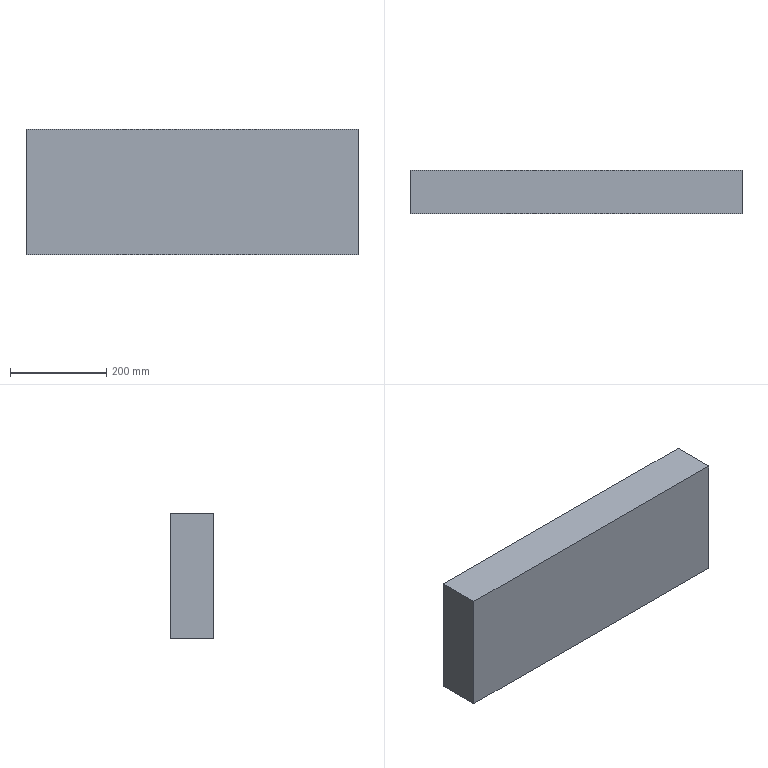Part | SolidWorks | features Extrusion 1, Shell 1 | 1 solid | 11 faces | box 690 x 90 x 260 mm | volume 2021904 mm3 | plane 11
STEP:
#1=CARTESIAN_POINT('',(345.,0.,130.));
#2=VERTEX_POINT('',#1);
#3=CARTESIAN_POINT('',(345.,0.,-130.));
#4=VERTEX_POINT('',#3);
#5=CARTESIAN_POINT('',(345.,0.,-130.));
#6=DIRECTION('',(0.,0.,-1.));
#7=VECTOR('',#6,1000.);
#8=LINE('',#5,#7);
#9=EDGE_CURVE('',#2,#4,#8,.T.);
#10=ORIENTED_EDGE('',*,*,#9,.T.);
#11=CARTESIAN_POINT('',(345.,90.,-130.));
#12=VERTEX_POINT('',#11);
#13=CARTESIAN_POINT('',(345.,90.,-130.));
#14=DIRECTION('',(0.,-1.,0.));
#15=VECTOR('',#14,1000.);
#16=LINE('',#13,#15);
#17=EDGE_CURVE('',#12,#4,#16,.T.);
#18=ORIENTED_EDGE('',*,*,#17,.F.);
#19=CARTESIAN_POINT('',(345.,90.,130.));
#20=VERTEX_POINT('',#19);
#21=CARTESIAN_POINT('',(345.,90.,-130.));
#22=DIRECTION('',(0.,0.,-1.));
#23=VECTOR('',#22,1000.);
#24=LINE('',#21,#23);
#25=EDGE_CURVE('',#20,#12,#24,.T.);
#26=ORIENTED_EDGE('',*,*,#25,.F.);
#27=CARTESIAN_POINT('',(345.,90.,130.));
#28=DIRECTION('',(0.,-1.,0.));
#29=VECTOR('',#28,1000.);
#30=LINE('',#27,#29);
#31=EDGE_CURVE('',#20,#2,#30,.T.);
#32=ORIENTED_EDGE('',*,*,#31,.T.);
#33=EDGE_LOOP('',(#10,#18,#26,#32));
#34=FACE_OUTER_BOUND('',#33,.T.);
#35=CARTESIAN_POINT('',(345.,90.,-130.));
#36=DIRECTION('',(-1.,0.,0.));
#37=DIRECTION('',(0.,0.,1.));
#38=AXIS2_PLACEMENT_3D('',#35,#36,#37);
#39=PLANE('',#38);
#40=ADVANCED_FACE('',(#34),#39,.F.);
#41=CARTESIAN_POINT('',(-345.,0.,-130.));
#42=VERTEX_POINT('',#41);
#43=CARTESIAN_POINT('',(-345.,0.,-130.));
#44=DIRECTION('',(-1.,0.,0.));
#45=VECTOR('',#44,1000.);
#46=LINE('',#43,#45);
#47=EDGE_CURVE('',#4,#42,#46,.T.);
#48=ORIENTED_EDGE('',*,*,#47,.T.);
#49=CARTESIAN_POINT('',(-345.,90.,-130.));
#50=VERTEX_POINT('',#49);
#51=CARTESIAN_POINT('',(-345.,90.,-130.));
#52=DIRECTION('',(0.,-1.,0.));
#53=VECTOR('',#52,1000.);
#54=LINE('',#51,#53);
#55=EDGE_CURVE('',#50,#42,#54,.T.);
#56=ORIENTED_EDGE('',*,*,#55,.F.);
#57=CARTESIAN_POINT('',(-345.,90.,-130.));
#58=DIRECTION('',(-1.,0.,0.));
#59=VECTOR('',#58,1000.);
#60=LINE('',#57,#59);
#61=EDGE_CURVE('',#12,#50,#60,.T.);
#62=ORIENTED_EDGE('',*,*,#61,.F.);
#63=ORIENTED_EDGE('',*,*,#17,.T.);
#64=EDGE_LOOP('',(#48,#56,#62,#63));
#65=FACE_OUTER_BOUND('',#64,.T.);
#66=CARTESIAN_POINT('',(-345.,90.,-130.));
#67=DIRECTION('',(0.,0.,1.));
#68=DIRECTION('',(1.,0.,0.));
#69=AXIS2_PLACEMENT_3D('',#66,#67,#68);
#70=PLANE('',#69);
#71=ADVANCED_FACE('',(#65),#70,.F.);
#72=CARTESIAN_POINT('',(-345.,0.,130.));
#73=VERTEX_POINT('',#72);
#74=CARTESIAN_POINT('',(-345.,0.,-130.));
#75=DIRECTION('',(0.,0.,1.));
#76=VECTOR('',#75,1000.);
#77=LINE('',#74,#76);
#78=EDGE_CURVE('',#42,#73,#77,.T.);
#79=ORIENTED_EDGE('',*,*,#78,.T.);
#80=CARTESIAN_POINT('',(-345.,90.,130.));
#81=VERTEX_POINT('',#80);
#82=CARTESIAN_POINT('',(-345.,90.,130.));
#83=DIRECTION('',(0.,-1.,0.));
#84=VECTOR('',#83,1000.);
#85=LINE('',#82,#84);
#86=EDGE_CURVE('',#81,#73,#85,.T.);
#87=ORIENTED_EDGE('',*,*,#86,.F.);
#88=CARTESIAN_POINT('',(-345.,90.,-130.));
#89=DIRECTION('',(0.,0.,1.));
#90=VECTOR('',#89,1000.);
#91=LINE('',#88,#90);
#92=EDGE_CURVE('',#50,#81,#91,.T.);
#93=ORIENTED_EDGE('',*,*,#92,.F.);
#94=ORIENTED_EDGE('',*,*,#55,.T.);
#95=EDGE_LOOP('',(#79,#87,#93,#94));
#96=FACE_OUTER_BOUND('',#95,.T.);
#97=CARTESIAN_POINT('',(-345.,90.,-130.));
#98=DIRECTION('',(1.,0.,0.));
#99=DIRECTION('',(0.,0.,-1.));
#100=AXIS2_PLACEMENT_3D('',#97,#98,#99);
#101=PLANE('',#100);
#102=ADVANCED_FACE('',(#96),#101,.F.);
#103=CARTESIAN_POINT('',(-345.,0.,130.));
#104=DIRECTION('',(1.,0.,0.));
#105=VECTOR('',#104,1000.);
#106=LINE('',#103,#105);
#107=EDGE_CURVE('',#73,#2,#106,.T.);
#108=ORIENTED_EDGE('',*,*,#107,.T.);
#109=ORIENTED_EDGE('',*,*,#31,.F.);
#110=CARTESIAN_POINT('',(-345.,90.,130.));
#111=DIRECTION('',(1.,0.,0.));
#112=VECTOR('',#111,1000.);
#113=LINE('',#110,#112);
#114=EDGE_CURVE('',#81,#20,#113,.T.);
#115=ORIENTED_EDGE('',*,*,#114,.F.);
#116=ORIENTED_EDGE('',*,*,#86,.T.);
#117=EDGE_LOOP('',(#108,#109,#115,#116));
#118=FACE_OUTER_BOUND('',#117,.T.);
#119=CARTESIAN_POINT('',(-345.,90.,130.));
#120=DIRECTION('',(0.,0.,-1.));
#121=DIRECTION('',(-1.,0.,0.));
#122=AXIS2_PLACEMENT_3D('',#119,#120,#121);
#123=PLANE('',#122);
#124=ADVANCED_FACE('',(#118),#123,.F.);
#125=CARTESIAN_POINT('',(339.,90.,124.));
#126=VERTEX_POINT('',#125);
#127=CARTESIAN_POINT('',(339.,90.,-124.));
#128=VERTEX_POINT('',#127);
#129=CARTESIAN_POINT('',(339.,90.,-130.));
#130=DIRECTION('',(0.,0.,-1.));
#131=VECTOR('',#130,1000.);
#132=LINE('',#129,#131);
#133=EDGE_CURVE('',#126,#128,#132,.T.);
#134=ORIENTED_EDGE('',*,*,#133,.F.);
#135=CARTESIAN_POINT('',(-339.,90.,124.));
#136=VERTEX_POINT('',#135);
#137=CARTESIAN_POINT('',(-345.,90.,124.));
#138=DIRECTION('',(1.,0.,0.));
#139=VECTOR('',#138,1000.);
#140=LINE('',#137,#139);
#141=EDGE_CURVE('',#136,#126,#140,.T.);
#142=ORIENTED_EDGE('',*,*,#141,.F.);
#143=CARTESIAN_POINT('',(-339.,90.,-124.));
#144=VERTEX_POINT('',#143);
#145=CARTESIAN_POINT('',(-339.,90.,-130.));
#146=DIRECTION('',(0.,0.,1.));
#147=VECTOR('',#146,1000.);
#148=LINE('',#145,#147);
#149=EDGE_CURVE('',#144,#136,#148,.T.);
#150=ORIENTED_EDGE('',*,*,#149,.F.);
#151=CARTESIAN_POINT('',(-345.,90.,-124.));
#152=DIRECTION('',(-1.,0.,0.));
#153=VECTOR('',#152,1000.);
#154=LINE('',#151,#153);
#155=EDGE_CURVE('',#128,#144,#154,.T.);
#156=ORIENTED_EDGE('',*,*,#155,.F.);
#157=EDGE_LOOP('',(#134,#142,#150,#156));
#158=FACE_BOUND('',#157,.T.);
#159=ORIENTED_EDGE('',*,*,#25,.T.);
#160=ORIENTED_EDGE('',*,*,#61,.T.);
#161=ORIENTED_EDGE('',*,*,#92,.T.);
#162=ORIENTED_EDGE('',*,*,#114,.T.);
#163=EDGE_LOOP('',(#159,#160,#161,#162));
#164=FACE_OUTER_BOUND('',#163,.T.);
#165=CARTESIAN_POINT('',(0.,90.,0.));
#166=DIRECTION('',(0.,1.,0.));
#167=DIRECTION('',(0.,0.,1.));
#168=AXIS2_PLACEMENT_3D('',#165,#166,#167);
#169=PLANE('',#168);
#170=ADVANCED_FACE('',(#158,#164),#169,.T.);
#171=ORIENTED_EDGE('',*,*,#9,.F.);
#172=ORIENTED_EDGE('',*,*,#107,.F.);
#173=ORIENTED_EDGE('',*,*,#78,.F.);
#174=ORIENTED_EDGE('',*,*,#47,.F.);
#175=EDGE_LOOP('',(#171,#172,#173,#174));
#176=FACE_OUTER_BOUND('',#175,.T.);
#177=CARTESIAN_POINT('',(0.,0.,0.));
#178=DIRECTION('',(0.,1.,0.));
#179=DIRECTION('',(0.,0.,1.));
#180=AXIS2_PLACEMENT_3D('',#177,#178,#179);
#181=PLANE('',#180);
#182=ADVANCED_FACE('',(#176),#181,.F.);
#183=CARTESIAN_POINT('',(339.,6.,124.));
#184=VERTEX_POINT('',#183);
#185=CARTESIAN_POINT('',(339.,6.,-124.));
#186=VERTEX_POINT('',#185);
#187=CARTESIAN_POINT('',(339.,6.,-130.));
#188=DIRECTION('',(0.,0.,-1.));
#189=VECTOR('',#188,1000.);
#190=LINE('',#187,#189);
#191=EDGE_CURVE('',#184,#186,#190,.T.);
#192=ORIENTED_EDGE('',*,*,#191,.F.);
#193=CARTESIAN_POINT('',(339.,90.,124.));
#194=DIRECTION('',(0.,-1.,0.));
#195=VECTOR('',#194,1000.);
#196=LINE('',#193,#195);
#197=EDGE_CURVE('',#126,#184,#196,.T.);
#198=ORIENTED_EDGE('',*,*,#197,.F.);
#199=ORIENTED_EDGE('',*,*,#133,.T.);
#200=CARTESIAN_POINT('',(339.,90.,-124.));
#201=DIRECTION('',(0.,-1.,0.));
#202=VECTOR('',#201,1000.);
#203=LINE('',#200,#202);
#204=EDGE_CURVE('',#128,#186,#203,.T.);
#205=ORIENTED_EDGE('',*,*,#204,.T.);
#206=EDGE_LOOP('',(#192,#198,#199,#205));
#207=FACE_OUTER_BOUND('',#206,.T.);
#208=CARTESIAN_POINT('',(339.,90.,-130.));
#209=DIRECTION('',(-1.,0.,0.));
#210=DIRECTION('',(0.,0.,1.));
#211=AXIS2_PLACEMENT_3D('',#208,#209,#210);
#212=PLANE('',#211);
#213=ADVANCED_FACE('',(#207),#212,.T.);
#214=CARTESIAN_POINT('',(-339.,6.,-124.));
#215=VERTEX_POINT('',#214);
#216=CARTESIAN_POINT('',(-345.,6.,-124.));
#217=DIRECTION('',(-1.,0.,0.));
#218=VECTOR('',#217,1000.);
#219=LINE('',#216,#218);
#220=EDGE_CURVE('',#186,#215,#219,.T.);
#221=ORIENTED_EDGE('',*,*,#220,.F.);
#222=ORIENTED_EDGE('',*,*,#204,.F.);
#223=ORIENTED_EDGE('',*,*,#155,.T.);
#224=CARTESIAN_POINT('',(-339.,90.,-124.));
#225=DIRECTION('',(0.,-1.,0.));
#226=VECTOR('',#225,1000.);
#227=LINE('',#224,#226);
#228=EDGE_CURVE('',#144,#215,#227,.T.);
#229=ORIENTED_EDGE('',*,*,#228,.T.);
#230=EDGE_LOOP('',(#221,#222,#223,#229));
#231=FACE_OUTER_BOUND('',#230,.T.);
#232=CARTESIAN_POINT('',(-345.,90.,-124.));
#233=DIRECTION('',(0.,0.,1.));
#234=DIRECTION('',(1.,0.,0.));
#235=AXIS2_PLACEMENT_3D('',#232,#233,#234);
#236=PLANE('',#235);
#237=ADVANCED_FACE('',(#231),#236,.T.);
#238=CARTESIAN_POINT('',(-339.,6.,124.));
#239=VERTEX_POINT('',#238);
#240=CARTESIAN_POINT('',(-339.,6.,-130.));
#241=DIRECTION('',(0.,0.,1.));
#242=VECTOR('',#241,1000.);
#243=LINE('',#240,#242);
#244=EDGE_CURVE('',#215,#239,#243,.T.);
#245=ORIENTED_EDGE('',*,*,#244,.F.);
#246=ORIENTED_EDGE('',*,*,#228,.F.);
#247=ORIENTED_EDGE('',*,*,#149,.T.);
#248=CARTESIAN_POINT('',(-339.,90.,124.));
#249=DIRECTION('',(0.,-1.,0.));
#250=VECTOR('',#249,1000.);
#251=LINE('',#248,#250);
#252=EDGE_CURVE('',#136,#239,#251,.T.);
#253=ORIENTED_EDGE('',*,*,#252,.T.);
#254=EDGE_LOOP('',(#245,#246,#247,#253));
#255=FACE_OUTER_BOUND('',#254,.T.);
#256=CARTESIAN_POINT('',(-339.,90.,-130.));
#257=DIRECTION('',(1.,0.,0.));
#258=DIRECTION('',(0.,0.,-1.));
#259=AXIS2_PLACEMENT_3D('',#256,#257,#258);
#260=PLANE('',#259);
#261=ADVANCED_FACE('',(#255),#260,.T.);
#262=CARTESIAN_POINT('',(-345.,6.,124.));
#263=DIRECTION('',(1.,0.,0.));
#264=VECTOR('',#263,1000.);
#265=LINE('',#262,#264);
#266=EDGE_CURVE('',#239,#184,#265,.T.);
#267=ORIENTED_EDGE('',*,*,#266,.F.);
#268=ORIENTED_EDGE('',*,*,#252,.F.);
#269=ORIENTED_EDGE('',*,*,#141,.T.);
#270=ORIENTED_EDGE('',*,*,#197,.T.);
#271=EDGE_LOOP('',(#267,#268,#269,#270));
#272=FACE_OUTER_BOUND('',#271,.T.);
#273=CARTESIAN_POINT('',(-345.,90.,124.));
#274=DIRECTION('',(0.,0.,-1.));
#275=DIRECTION('',(-1.,0.,0.));
#276=AXIS2_PLACEMENT_3D('',#273,#274,#275);
#277=PLANE('',#276);
#278=ADVANCED_FACE('',(#272),#277,.T.);
#279=ORIENTED_EDGE('',*,*,#191,.T.);
#280=ORIENTED_EDGE('',*,*,#220,.T.);
#281=ORIENTED_EDGE('',*,*,#244,.T.);
#282=ORIENTED_EDGE('',*,*,#266,.T.);
#283=EDGE_LOOP('',(#279,#280,#281,#282));
#284=FACE_OUTER_BOUND('',#283,.T.);
#285=CARTESIAN_POINT('',(0.,6.,0.));
#286=DIRECTION('',(0.,1.,0.));
#287=DIRECTION('',(0.,0.,1.));
#288=AXIS2_PLACEMENT_3D('',#285,#286,#287);
#289=PLANE('',#288);
#290=ADVANCED_FACE('',(#284),#289,.T.);
#291=CLOSED_SHELL('',(#40,#71,#102,#124,#170,#182,#213,#237,#261,#278,#290));
#292=MANIFOLD_SOLID_BREP('',#291);
#293=CARTESIAN_POINT('',(0.,0.,0.));
#294=DIRECTION('',(0.,0.,1.));
#295=DIRECTION('',(1.,0.,0.));
#296=AXIS2_PLACEMENT_3D('',#293,#294,#295);
#297=(LENGTH_UNIT()NAMED_UNIT(*)SI_UNIT(.MILLI.,.METRE.));
#298=UNCERTAINTY_MEASURE_WITH_UNIT(LENGTH_MEASURE(0.00001),#297,'','');
#299=(NAMED_UNIT(*)PLANE_ANGLE_UNIT()SI_UNIT($,.RADIAN.));
#300=(NAMED_UNIT(*)SI_UNIT($,.STERADIAN.)SOLID_ANGLE_UNIT());
#301=(GEOMETRIC_REPRESENTATION_CONTEXT(3)GLOBAL_UNCERTAINTY_ASSIGNED_CONTEXT((#298))GLOBAL_UNIT_ASSIGNED_CONTEXT((#297,#299,#300))REPRESENTATION_CONTEXT('',''));
#302=ADVANCED_BREP_SHAPE_REPRESENTATION('',(#292,#296),#301);